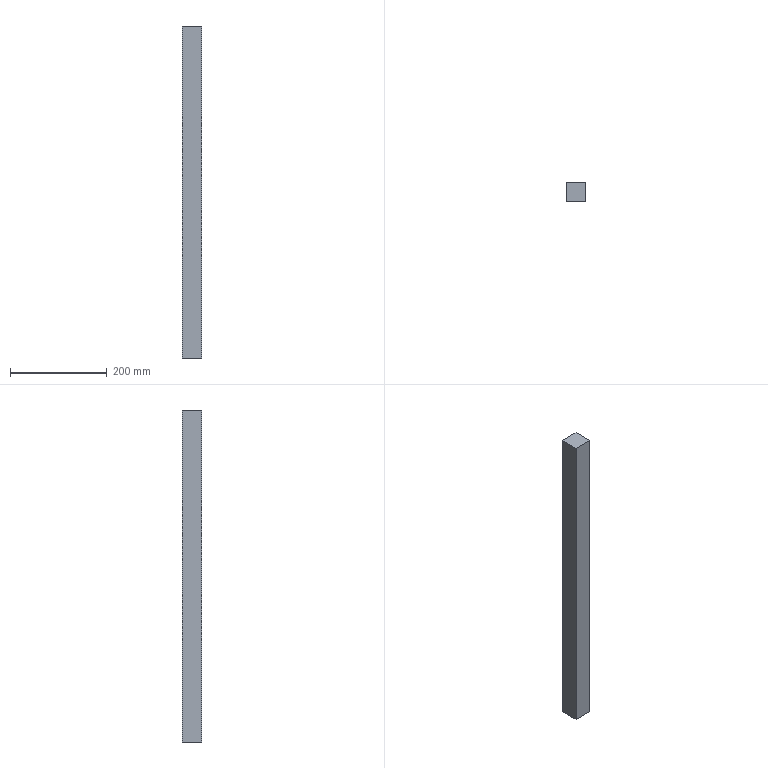Part | NX | 1 solid | 6 faces | box 40 x 40 x 684.8 mm | volume 1095680 mm3 | plane 6
STEP:
#1=CARTESIAN_POINT('',(-409.726,88.985,0.));
#2=VERTEX_POINT('',#1);
#3=CARTESIAN_POINT('',(-369.726,88.985,0.));
#4=VERTEX_POINT('',#3);
#5=CARTESIAN_POINT('',(30.669,88.985,0.));
#6=DIRECTION('',(1.,0.,0.));
#7=VECTOR('',#6,1000.);
#8=LINE('',#5,#7);
#9=EDGE_CURVE('',#2,#4,#8,.T.);
#10=ORIENTED_EDGE('',*,*,#9,.T.);
#11=CARTESIAN_POINT('',(-369.726,88.985,-684.8));
#12=VERTEX_POINT('',#11);
#13=CARTESIAN_POINT('',(-369.726,88.985,0.));
#14=DIRECTION('',(0.,0.,-1.));
#15=VECTOR('',#14,1000.);
#16=LINE('',#13,#15);
#17=EDGE_CURVE('',#4,#12,#16,.T.);
#18=ORIENTED_EDGE('',*,*,#17,.T.);
#19=CARTESIAN_POINT('',(-409.726,88.985,-684.8));
#20=VERTEX_POINT('',#19);
#21=CARTESIAN_POINT('',(0.,88.985,-684.8));
#22=DIRECTION('',(1.,0.,0.));
#23=VECTOR('',#22,1000.);
#24=LINE('',#21,#23);
#25=EDGE_CURVE('',#20,#12,#24,.T.);
#26=ORIENTED_EDGE('',*,*,#25,.F.);
#27=CARTESIAN_POINT('',(-409.726,88.985,0.));
#28=DIRECTION('',(0.,0.,-1.));
#29=VECTOR('',#28,1000.);
#30=LINE('',#27,#29);
#31=EDGE_CURVE('',#2,#20,#30,.T.);
#32=ORIENTED_EDGE('',*,*,#31,.F.);
#33=EDGE_LOOP('',(#10,#18,#26,#32));
#34=FACE_BOUND('',#33,.T.);
#35=CARTESIAN_POINT('',(-369.726,88.985,0.));
#36=DIRECTION('',(0.,1.,0.));
#37=DIRECTION('',(1.,0.,0.));
#38=AXIS2_PLACEMENT_3D('',#35,#36,#37);
#39=PLANE('',#38);
#40=ADVANCED_FACE('',(#34),#39,.T.);
#41=CARTESIAN_POINT('',(-369.726,48.985,0.));
#42=VERTEX_POINT('',#41);
#43=CARTESIAN_POINT('',(-369.726,88.985,0.));
#44=DIRECTION('',(0.,-1.,0.));
#45=VECTOR('',#44,1000.);
#46=LINE('',#43,#45);
#47=EDGE_CURVE('',#4,#42,#46,.T.);
#48=ORIENTED_EDGE('',*,*,#47,.T.);
#49=CARTESIAN_POINT('',(-369.726,48.985,-684.8));
#50=VERTEX_POINT('',#49);
#51=CARTESIAN_POINT('',(-369.726,48.985,0.));
#52=DIRECTION('',(0.,0.,-1.));
#53=VECTOR('',#52,1000.);
#54=LINE('',#51,#53);
#55=EDGE_CURVE('',#42,#50,#54,.T.);
#56=ORIENTED_EDGE('',*,*,#55,.T.);
#57=CARTESIAN_POINT('',(-369.726,0.,-684.8));
#58=DIRECTION('',(0.,-1.,0.));
#59=VECTOR('',#58,1000.);
#60=LINE('',#57,#59);
#61=EDGE_CURVE('',#12,#50,#60,.T.);
#62=ORIENTED_EDGE('',*,*,#61,.F.);
#63=ORIENTED_EDGE('',*,*,#17,.F.);
#64=EDGE_LOOP('',(#48,#56,#62,#63));
#65=FACE_BOUND('',#64,.T.);
#66=CARTESIAN_POINT('',(-369.726,48.985,0.));
#67=DIRECTION('',(1.,0.,0.));
#68=DIRECTION('',(0.,1.,0.));
#69=AXIS2_PLACEMENT_3D('',#66,#67,#68);
#70=PLANE('',#69);
#71=ADVANCED_FACE('',(#65),#70,.T.);
#72=CARTESIAN_POINT('',(-409.726,48.985,0.));
#73=VERTEX_POINT('',#72);
#74=CARTESIAN_POINT('',(-409.726,48.985,0.));
#75=DIRECTION('',(1.,0.,0.));
#76=VECTOR('',#75,1000.);
#77=LINE('',#74,#76);
#78=EDGE_CURVE('',#73,#42,#77,.T.);
#79=ORIENTED_EDGE('',*,*,#78,.F.);
#80=CARTESIAN_POINT('',(-409.726,48.985,-684.8));
#81=VERTEX_POINT('',#80);
#82=CARTESIAN_POINT('',(-409.726,48.985,0.));
#83=DIRECTION('',(0.,0.,-1.));
#84=VECTOR('',#83,1000.);
#85=LINE('',#82,#84);
#86=EDGE_CURVE('',#73,#81,#85,.T.);
#87=ORIENTED_EDGE('',*,*,#86,.T.);
#88=CARTESIAN_POINT('',(0.,48.985,-684.8));
#89=DIRECTION('',(-1.,0.,0.));
#90=VECTOR('',#89,1000.);
#91=LINE('',#88,#90);
#92=EDGE_CURVE('',#50,#81,#91,.T.);
#93=ORIENTED_EDGE('',*,*,#92,.F.);
#94=ORIENTED_EDGE('',*,*,#55,.F.);
#95=EDGE_LOOP('',(#79,#87,#93,#94));
#96=FACE_BOUND('',#95,.T.);
#97=CARTESIAN_POINT('',(-409.726,48.985,0.));
#98=DIRECTION('',(0.,-1.,0.));
#99=DIRECTION('',(0.,0.,-1.));
#100=AXIS2_PLACEMENT_3D('',#97,#98,#99);
#101=PLANE('',#100);
#102=ADVANCED_FACE('',(#96),#101,.T.);
#103=CARTESIAN_POINT('',(-409.726,88.985,0.));
#104=DIRECTION('',(0.,-1.,0.));
#105=VECTOR('',#104,1000.);
#106=LINE('',#103,#105);
#107=EDGE_CURVE('',#2,#73,#106,.T.);
#108=ORIENTED_EDGE('',*,*,#107,.F.);
#109=ORIENTED_EDGE('',*,*,#31,.T.);
#110=CARTESIAN_POINT('',(-409.726,0.,-684.8));
#111=DIRECTION('',(0.,1.,0.));
#112=VECTOR('',#111,1000.);
#113=LINE('',#110,#112);
#114=EDGE_CURVE('',#81,#20,#113,.T.);
#115=ORIENTED_EDGE('',*,*,#114,.F.);
#116=ORIENTED_EDGE('',*,*,#86,.F.);
#117=EDGE_LOOP('',(#108,#109,#115,#116));
#118=FACE_BOUND('',#117,.T.);
#119=CARTESIAN_POINT('',(-409.726,88.985,0.));
#120=DIRECTION('',(-1.,0.,0.));
#121=DIRECTION('',(0.,0.,1.));
#122=AXIS2_PLACEMENT_3D('',#119,#120,#121);
#123=PLANE('',#122);
#124=ADVANCED_FACE('',(#118),#123,.T.);
#125=ORIENTED_EDGE('',*,*,#92,.T.);
#126=ORIENTED_EDGE('',*,*,#114,.T.);
#127=ORIENTED_EDGE('',*,*,#25,.T.);
#128=ORIENTED_EDGE('',*,*,#61,.T.);
#129=EDGE_LOOP('',(#125,#126,#127,#128));
#130=FACE_BOUND('',#129,.T.);
#131=CARTESIAN_POINT('',(0.,0.,-684.8));
#132=DIRECTION('',(0.,0.,1.));
#133=DIRECTION('',(1.,0.,0.));
#134=AXIS2_PLACEMENT_3D('',#131,#132,#133);
#135=PLANE('',#134);
#136=ADVANCED_FACE('',(#130),#135,.F.);
#137=ORIENTED_EDGE('',*,*,#47,.F.);
#138=ORIENTED_EDGE('',*,*,#9,.F.);
#139=ORIENTED_EDGE('',*,*,#107,.T.);
#140=ORIENTED_EDGE('',*,*,#78,.T.);
#141=EDGE_LOOP('',(#137,#138,#139,#140));
#142=FACE_BOUND('',#141,.T.);
#143=CARTESIAN_POINT('',(0.,0.,0.));
#144=DIRECTION('',(0.,0.,1.));
#145=DIRECTION('',(1.,0.,0.));
#146=AXIS2_PLACEMENT_3D('',#143,#144,#145);
#147=PLANE('',#146);
#148=ADVANCED_FACE('',(#142),#147,.T.);
#149=CLOSED_SHELL('',(#40,#71,#102,#124,#136,#148));
#150=MANIFOLD_SOLID_BREP('',#149);
#151=(LENGTH_UNIT()NAMED_UNIT(*)SI_UNIT(.MILLI.,.METRE.));
#152=UNCERTAINTY_MEASURE_WITH_UNIT(LENGTH_MEASURE(0.00001),#151,'','');
#153=(NAMED_UNIT(*)PLANE_ANGLE_UNIT()SI_UNIT($,.RADIAN.));
#154=(NAMED_UNIT(*)SI_UNIT($,.STERADIAN.)SOLID_ANGLE_UNIT());
#155=(GEOMETRIC_REPRESENTATION_CONTEXT(3)GLOBAL_UNCERTAINTY_ASSIGNED_CONTEXT((#152))GLOBAL_UNIT_ASSIGNED_CONTEXT((#151,#153,#154))REPRESENTATION_CONTEXT('',''));
#156=ADVANCED_BREP_SHAPE_REPRESENTATION('',(#150),#155);